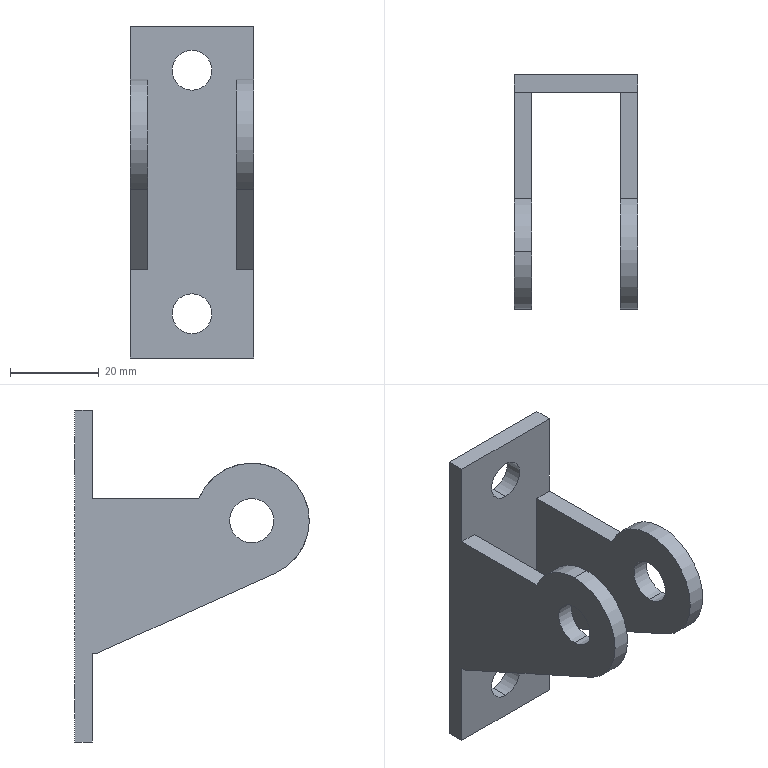Part | SolidWorks | features BaseBody 1 | 1 solid | 25 faces | box 28 x 53 x 75 mm | volume 17835 mm3 | plane 14 | cylinder 11 | commonest cylinder face diameters 9 x4 10 x4 26 x3
STEP:
#1=CARTESIAN_POINT('',(-400.,2358.,-1337.));
#2=VERTEX_POINT('',#1);
#3=CARTESIAN_POINT('',(-400.,2358.,-1328.));
#4=VERTEX_POINT('',#3);
#5=CARTESIAN_POINT('',(-400.,2358.,-1332.5));
#6=DIRECTION('',(0.,1.,0.));
#7=DIRECTION('',(0.,0.,1.));
#8=AXIS2_PLACEMENT_3D('',#5,#6,#7);
#9=CIRCLE('',#8,4.5);
#10=EDGE_CURVE('',#2,#4,#9,.T.);
#11=ORIENTED_EDGE('',*,*,#10,.F.);
#12=CARTESIAN_POINT('',(-400.,2362.,-1337.));
#13=VERTEX_POINT('',#12);
#14=CARTESIAN_POINT('',(-400.,2362.,-1337.));
#15=DIRECTION('',(0.,1.,0.));
#16=VECTOR('',#15,1000.);
#17=LINE('',#14,#16);
#18=EDGE_CURVE('',#2,#13,#17,.T.);
#19=ORIENTED_EDGE('',*,*,#18,.T.);
#20=CARTESIAN_POINT('',(-400.,2362.,-1328.));
#21=VERTEX_POINT('',#20);
#22=CARTESIAN_POINT('',(-400.,2362.,-1332.5));
#23=DIRECTION('',(0.,1.,0.));
#24=DIRECTION('',(0.,0.,1.));
#25=AXIS2_PLACEMENT_3D('',#22,#23,#24);
#26=CIRCLE('',#25,4.5);
#27=EDGE_CURVE('',#13,#21,#26,.T.);
#28=ORIENTED_EDGE('',*,*,#27,.T.);
#29=CARTESIAN_POINT('',(-400.,2362.,-1328.));
#30=DIRECTION('',(0.,1.,0.));
#31=VECTOR('',#30,1000.);
#32=LINE('',#29,#31);
#33=EDGE_CURVE('',#4,#21,#32,.T.);
#34=ORIENTED_EDGE('',*,*,#33,.F.);
#35=EDGE_LOOP('',(#11,#19,#28,#34));
#36=FACE_OUTER_BOUND('',#35,.T.);
#37=CARTESIAN_POINT('',(-400.,2362.,-1332.5));
#38=DIRECTION('',(0.,1.,0.));
#39=DIRECTION('',(0.,0.,1.));
#40=AXIS2_PLACEMENT_3D('',#37,#38,#39);
#41=CYLINDRICAL_SURFACE('',#40,4.5);
#42=ADVANCED_FACE('',(#36),#41,.F.);
#43=CARTESIAN_POINT('',(-400.,2362.,-1282.));
#44=VERTEX_POINT('',#43);
#45=CARTESIAN_POINT('',(-400.,2362.,-1273.));
#46=VERTEX_POINT('',#45);
#47=CARTESIAN_POINT('',(-400.,2362.,-1277.5));
#48=DIRECTION('',(0.,1.,0.));
#49=DIRECTION('',(0.,0.,-1.));
#50=AXIS2_PLACEMENT_3D('',#47,#48,#49);
#51=CIRCLE('',#50,4.5);
#52=EDGE_CURVE('',#44,#46,#51,.T.);
#53=ORIENTED_EDGE('',*,*,#52,.T.);
#54=CARTESIAN_POINT('',(-400.,2358.,-1273.));
#55=VERTEX_POINT('',#54);
#56=CARTESIAN_POINT('',(-400.,2362.,-1273.));
#57=DIRECTION('',(0.,-1.,0.));
#58=VECTOR('',#57,1000.);
#59=LINE('',#56,#58);
#60=EDGE_CURVE('',#46,#55,#59,.T.);
#61=ORIENTED_EDGE('',*,*,#60,.T.);
#62=CARTESIAN_POINT('',(-400.,2358.,-1282.));
#63=VERTEX_POINT('',#62);
#64=CARTESIAN_POINT('',(-400.,2358.,-1277.5));
#65=DIRECTION('',(0.,1.,0.));
#66=DIRECTION('',(0.,0.,-1.));
#67=AXIS2_PLACEMENT_3D('',#64,#65,#66);
#68=CIRCLE('',#67,4.5);
#69=EDGE_CURVE('',#63,#55,#68,.T.);
#70=ORIENTED_EDGE('',*,*,#69,.F.);
#71=CARTESIAN_POINT('',(-400.,2362.,-1282.));
#72=DIRECTION('',(0.,-1.,0.));
#73=VECTOR('',#72,1000.);
#74=LINE('',#71,#73);
#75=EDGE_CURVE('',#44,#63,#74,.T.);
#76=ORIENTED_EDGE('',*,*,#75,.F.);
#77=EDGE_LOOP('',(#53,#61,#70,#76));
#78=FACE_OUTER_BOUND('',#77,.T.);
#79=CARTESIAN_POINT('',(-400.,2362.,-1277.5));
#80=DIRECTION('',(0.,-1.,0.));
#81=DIRECTION('',(0.,0.,-1.));
#82=AXIS2_PLACEMENT_3D('',#79,#80,#81);
#83=CYLINDRICAL_SURFACE('',#82,4.5);
#84=ADVANCED_FACE('',(#78),#83,.F.);
#85=CARTESIAN_POINT('',(-410.,2322.,-1297.5));
#86=VERTEX_POINT('',#85);
#87=CARTESIAN_POINT('',(-410.,2322.,-1287.5));
#88=VERTEX_POINT('',#87);
#89=CARTESIAN_POINT('',(-410.,2322.,-1292.5));
#90=DIRECTION('',(-1.,0.,0.));
#91=DIRECTION('',(0.,0.,1.));
#92=AXIS2_PLACEMENT_3D('',#89,#90,#91);
#93=CIRCLE('',#92,5.);
#94=EDGE_CURVE('',#86,#88,#93,.T.);
#95=ORIENTED_EDGE('',*,*,#94,.F.);
#96=CARTESIAN_POINT('',(-414.,2322.,-1297.5));
#97=VERTEX_POINT('',#96);
#98=CARTESIAN_POINT('',(-414.,2322.,-1297.5));
#99=DIRECTION('',(-1.,0.,0.));
#100=VECTOR('',#99,1000.);
#101=LINE('',#98,#100);
#102=EDGE_CURVE('',#86,#97,#101,.T.);
#103=ORIENTED_EDGE('',*,*,#102,.T.);
#104=CARTESIAN_POINT('',(-414.,2322.,-1287.5));
#105=VERTEX_POINT('',#104);
#106=CARTESIAN_POINT('',(-414.,2322.,-1292.5));
#107=DIRECTION('',(1.,0.,0.));
#108=DIRECTION('',(0.,0.,1.));
#109=AXIS2_PLACEMENT_3D('',#106,#107,#108);
#110=CIRCLE('',#109,5.);
#111=EDGE_CURVE('',#105,#97,#110,.T.);
#112=ORIENTED_EDGE('',*,*,#111,.F.);
#113=CARTESIAN_POINT('',(-414.,2322.,-1287.5));
#114=DIRECTION('',(-1.,0.,0.));
#115=VECTOR('',#114,1000.);
#116=LINE('',#113,#115);
#117=EDGE_CURVE('',#88,#105,#116,.T.);
#118=ORIENTED_EDGE('',*,*,#117,.F.);
#119=EDGE_LOOP('',(#95,#103,#112,#118));
#120=FACE_OUTER_BOUND('',#119,.T.);
#121=CARTESIAN_POINT('',(-414.,2322.,-1292.5));
#122=DIRECTION('',(-1.,0.,0.));
#123=DIRECTION('',(0.,0.,1.));
#124=AXIS2_PLACEMENT_3D('',#121,#122,#123);
#125=CYLINDRICAL_SURFACE('',#124,5.);
#126=ADVANCED_FACE('',(#120),#125,.F.);
#127=CARTESIAN_POINT('',(-410.,2316.667,-1304.356));
#128=VERTEX_POINT('',#127);
#129=CARTESIAN_POINT('',(-410.,2322.,-1279.5));
#130=VERTEX_POINT('',#129);
#131=CARTESIAN_POINT('',(-410.,2322.,-1292.5));
#132=DIRECTION('',(-1.,0.,0.));
#133=DIRECTION('',(0.,0.,1.));
#134=AXIS2_PLACEMENT_3D('',#131,#132,#133);
#135=CIRCLE('',#134,13.);
#136=EDGE_CURVE('',#128,#130,#135,.T.);
#137=ORIENTED_EDGE('',*,*,#136,.T.);
#138=CARTESIAN_POINT('',(-414.,2322.,-1279.5));
#139=VERTEX_POINT('',#138);
#140=CARTESIAN_POINT('',(-414.,2322.,-1279.5));
#141=DIRECTION('',(-1.,0.,0.));
#142=VECTOR('',#141,1000.);
#143=LINE('',#140,#142);
#144=EDGE_CURVE('',#130,#139,#143,.T.);
#145=ORIENTED_EDGE('',*,*,#144,.T.);
#146=CARTESIAN_POINT('',(-414.,2316.667,-1304.356));
#147=VERTEX_POINT('',#146);
#148=CARTESIAN_POINT('',(-414.,2322.,-1292.5));
#149=DIRECTION('',(-1.,0.,0.));
#150=DIRECTION('',(0.,0.,1.));
#151=AXIS2_PLACEMENT_3D('',#148,#149,#150);
#152=CIRCLE('',#151,13.);
#153=EDGE_CURVE('',#147,#139,#152,.T.);
#154=ORIENTED_EDGE('',*,*,#153,.F.);
#155=CARTESIAN_POINT('',(-414.,2316.667,-1304.356));
#156=DIRECTION('',(1.,0.,0.));
#157=VECTOR('',#156,1000.);
#158=LINE('',#155,#157);
#159=EDGE_CURVE('',#147,#128,#158,.T.);
#160=ORIENTED_EDGE('',*,*,#159,.T.);
#161=EDGE_LOOP('',(#137,#145,#154,#160));
#162=FACE_OUTER_BOUND('',#161,.T.);
#163=CARTESIAN_POINT('',(-414.,2322.,-1292.5));
#164=DIRECTION('',(-1.,0.,0.));
#165=DIRECTION('',(0.,0.,1.));
#166=AXIS2_PLACEMENT_3D('',#163,#164,#165);
#167=CYLINDRICAL_SURFACE('',#166,13.);
#168=ADVANCED_FACE('',(#162),#167,.T.);
#169=CARTESIAN_POINT('',(-390.,2322.,-1287.5));
#170=VERTEX_POINT('',#169);
#171=CARTESIAN_POINT('',(-390.,2322.,-1297.5));
#172=VERTEX_POINT('',#171);
#173=CARTESIAN_POINT('',(-390.,2322.,-1292.5));
#174=DIRECTION('',(1.,0.,0.));
#175=DIRECTION('',(0.,0.,-1.));
#176=AXIS2_PLACEMENT_3D('',#173,#174,#175);
#177=CIRCLE('',#176,5.);
#178=EDGE_CURVE('',#170,#172,#177,.T.);
#179=ORIENTED_EDGE('',*,*,#178,.F.);
#180=CARTESIAN_POINT('',(-386.,2322.,-1287.5));
#181=VERTEX_POINT('',#180);
#182=CARTESIAN_POINT('',(-386.,2322.,-1287.5));
#183=DIRECTION('',(1.,0.,0.));
#184=VECTOR('',#183,1000.);
#185=LINE('',#182,#184);
#186=EDGE_CURVE('',#170,#181,#185,.T.);
#187=ORIENTED_EDGE('',*,*,#186,.T.);
#188=CARTESIAN_POINT('',(-386.,2322.,-1297.5));
#189=VERTEX_POINT('',#188);
#190=CARTESIAN_POINT('',(-386.,2322.,-1292.5));
#191=DIRECTION('',(-1.,0.,0.));
#192=DIRECTION('',(0.,0.,-1.));
#193=AXIS2_PLACEMENT_3D('',#190,#191,#192);
#194=CIRCLE('',#193,5.);
#195=EDGE_CURVE('',#189,#181,#194,.T.);
#196=ORIENTED_EDGE('',*,*,#195,.F.);
#197=CARTESIAN_POINT('',(-386.,2322.,-1297.5));
#198=DIRECTION('',(1.,0.,0.));
#199=VECTOR('',#198,1000.);
#200=LINE('',#197,#199);
#201=EDGE_CURVE('',#172,#189,#200,.T.);
#202=ORIENTED_EDGE('',*,*,#201,.F.);
#203=EDGE_LOOP('',(#179,#187,#196,#202));
#204=FACE_OUTER_BOUND('',#203,.T.);
#205=CARTESIAN_POINT('',(-386.,2322.,-1292.5));
#206=DIRECTION('',(1.,0.,0.));
#207=DIRECTION('',(0.,0.,-1.));
#208=AXIS2_PLACEMENT_3D('',#205,#206,#207);
#209=CYLINDRICAL_SURFACE('',#208,5.);
#210=ADVANCED_FACE('',(#204),#209,.F.);
#211=CARTESIAN_POINT('',(-400.,2362.,-1332.5));
#212=DIRECTION('',(0.,1.,0.));
#213=DIRECTION('',(0.,0.,1.));
#214=AXIS2_PLACEMENT_3D('',#211,#212,#213);
#215=CIRCLE('',#214,4.5);
#216=EDGE_CURVE('',#21,#13,#215,.T.);
#217=ORIENTED_EDGE('',*,*,#216,.F.);
#218=ORIENTED_EDGE('',*,*,#27,.F.);
#219=EDGE_LOOP('',(#217,#218));
#220=FACE_BOUND('',#219,.T.);
#221=ORIENTED_EDGE('',*,*,#52,.F.);
#222=CARTESIAN_POINT('',(-400.,2362.,-1277.5));
#223=DIRECTION('',(0.,1.,0.));
#224=DIRECTION('',(0.,0.,-1.));
#225=AXIS2_PLACEMENT_3D('',#222,#223,#224);
#226=CIRCLE('',#225,4.5);
#227=EDGE_CURVE('',#46,#44,#226,.T.);
#228=ORIENTED_EDGE('',*,*,#227,.F.);
#229=EDGE_LOOP('',(#221,#228));
#230=FACE_BOUND('',#229,.T.);
#231=CARTESIAN_POINT('',(-386.,2362.,-1267.5));
#232=VERTEX_POINT('',#231);
#233=CARTESIAN_POINT('',(-414.,2362.,-1267.5));
#234=VERTEX_POINT('',#233);
#235=CARTESIAN_POINT('',(-400.,2362.,-1267.5));
#236=DIRECTION('',(-1.,0.,0.));
#237=VECTOR('',#236,1000.);
#238=LINE('',#235,#237);
#239=EDGE_CURVE('',#232,#234,#238,.T.);
#240=ORIENTED_EDGE('',*,*,#239,.F.);
#241=CARTESIAN_POINT('',(-386.,2362.,-1342.5));
#242=VERTEX_POINT('',#241);
#243=CARTESIAN_POINT('',(-386.,2362.,-1292.5));
#244=DIRECTION('',(0.,0.,1.));
#245=VECTOR('',#244,1000.);
#246=LINE('',#243,#245);
#247=EDGE_CURVE('',#242,#232,#246,.T.);
#248=ORIENTED_EDGE('',*,*,#247,.F.);
#249=CARTESIAN_POINT('',(-414.,2362.,-1342.5));
#250=VERTEX_POINT('',#249);
#251=CARTESIAN_POINT('',(-400.,2362.,-1342.5));
#252=DIRECTION('',(1.,0.,0.));
#253=VECTOR('',#252,1000.);
#254=LINE('',#251,#253);
#255=EDGE_CURVE('',#250,#242,#254,.T.);
#256=ORIENTED_EDGE('',*,*,#255,.F.);
#257=CARTESIAN_POINT('',(-414.,2362.,-1292.5));
#258=DIRECTION('',(0.,0.,-1.));
#259=VECTOR('',#258,1000.);
#260=LINE('',#257,#259);
#261=EDGE_CURVE('',#234,#250,#260,.T.);
#262=ORIENTED_EDGE('',*,*,#261,.F.);
#263=EDGE_LOOP('',(#240,#248,#256,#262));
#264=FACE_OUTER_BOUND('',#263,.T.);
#265=CARTESIAN_POINT('',(-400.,2362.,-1292.5));
#266=DIRECTION('',(0.,-1.,0.));
#267=DIRECTION('',(0.,0.,-1.));
#268=AXIS2_PLACEMENT_3D('',#265,#266,#267);
#269=PLANE('',#268);
#270=ADVANCED_FACE('',(#220,#230,#264),#269,.F.);
#271=ORIENTED_EDGE('',*,*,#18,.F.);
#272=CARTESIAN_POINT('',(-400.,2358.,-1332.5));
#273=DIRECTION('',(0.,1.,0.));
#274=DIRECTION('',(0.,0.,1.));
#275=AXIS2_PLACEMENT_3D('',#272,#273,#274);
#276=CIRCLE('',#275,4.5);
#277=EDGE_CURVE('',#4,#2,#276,.T.);
#278=ORIENTED_EDGE('',*,*,#277,.F.);
#279=ORIENTED_EDGE('',*,*,#33,.T.);
#280=ORIENTED_EDGE('',*,*,#216,.T.);
#281=EDGE_LOOP('',(#271,#278,#279,#280));
#282=FACE_OUTER_BOUND('',#281,.T.);
#283=CARTESIAN_POINT('',(-400.,2362.,-1332.5));
#284=DIRECTION('',(0.,1.,0.));
#285=DIRECTION('',(0.,0.,1.));
#286=AXIS2_PLACEMENT_3D('',#283,#284,#285);
#287=CYLINDRICAL_SURFACE('',#286,4.5);
#288=ADVANCED_FACE('',(#282),#287,.F.);
#289=ORIENTED_EDGE('',*,*,#60,.F.);
#290=ORIENTED_EDGE('',*,*,#227,.T.);
#291=ORIENTED_EDGE('',*,*,#75,.T.);
#292=CARTESIAN_POINT('',(-400.,2358.,-1277.5));
#293=DIRECTION('',(0.,1.,0.));
#294=DIRECTION('',(0.,0.,-1.));
#295=AXIS2_PLACEMENT_3D('',#292,#293,#294);
#296=CIRCLE('',#295,4.5);
#297=EDGE_CURVE('',#55,#63,#296,.T.);
#298=ORIENTED_EDGE('',*,*,#297,.F.);
#299=EDGE_LOOP('',(#289,#290,#291,#298));
#300=FACE_OUTER_BOUND('',#299,.T.);
#301=CARTESIAN_POINT('',(-400.,2362.,-1277.5));
#302=DIRECTION('',(0.,-1.,0.));
#303=DIRECTION('',(0.,0.,-1.));
#304=AXIS2_PLACEMENT_3D('',#301,#302,#303);
#305=CYLINDRICAL_SURFACE('',#304,4.5);
#306=ADVANCED_FACE('',(#300),#305,.F.);
#307=ORIENTED_EDGE('',*,*,#111,.T.);
#308=CARTESIAN_POINT('',(-414.,2322.,-1292.5));
#309=DIRECTION('',(1.,0.,0.));
#310=DIRECTION('',(0.,0.,1.));
#311=AXIS2_PLACEMENT_3D('',#308,#309,#310);
#312=CIRCLE('',#311,5.);
#313=EDGE_CURVE('',#97,#105,#312,.T.);
#314=ORIENTED_EDGE('',*,*,#313,.T.);
#315=EDGE_LOOP('',(#307,#314));
#316=FACE_BOUND('',#315,.T.);
#317=CARTESIAN_POINT('',(-414.,2334.,-1287.5));
#318=VERTEX_POINT('',#317);
#319=CARTESIAN_POINT('',(-414.,2358.,-1287.5));
#320=VERTEX_POINT('',#319);
#321=CARTESIAN_POINT('',(-414.,2362.,-1287.5));
#322=DIRECTION('',(0.,1.,0.));
#323=VECTOR('',#322,1000.);
#324=LINE('',#321,#323);
#325=EDGE_CURVE('',#318,#320,#324,.T.);
#326=ORIENTED_EDGE('',*,*,#325,.T.);
#327=CARTESIAN_POINT('',(-414.,2358.,-1267.5));
#328=VERTEX_POINT('',#327);
#329=CARTESIAN_POINT('',(-414.,2358.,-1342.5));
#330=DIRECTION('',(0.,0.,1.));
#331=VECTOR('',#330,1000.);
#332=LINE('',#329,#331);
#333=EDGE_CURVE('',#320,#328,#332,.T.);
#334=ORIENTED_EDGE('',*,*,#333,.T.);
#335=CARTESIAN_POINT('',(-414.,2362.,-1267.5));
#336=DIRECTION('',(0.,1.,0.));
#337=VECTOR('',#336,1000.);
#338=LINE('',#335,#337);
#339=EDGE_CURVE('',#328,#234,#338,.T.);
#340=ORIENTED_EDGE('',*,*,#339,.T.);
#341=ORIENTED_EDGE('',*,*,#261,.T.);
#342=CARTESIAN_POINT('',(-414.,2358.,-1342.5));
#343=VERTEX_POINT('',#342);
#344=CARTESIAN_POINT('',(-414.,2362.,-1342.5));
#345=DIRECTION('',(0.,-1.,0.));
#346=VECTOR('',#345,1000.);
#347=LINE('',#344,#346);
#348=EDGE_CURVE('',#250,#343,#347,.T.);
#349=ORIENTED_EDGE('',*,*,#348,.T.);
#350=CARTESIAN_POINT('',(-414.,2358.,-1322.5));
#351=VERTEX_POINT('',#350);
#352=CARTESIAN_POINT('',(-414.,2358.,-1342.5));
#353=DIRECTION('',(0.,0.,1.));
#354=VECTOR('',#353,1000.);
#355=LINE('',#352,#354);
#356=EDGE_CURVE('',#343,#351,#355,.T.);
#357=ORIENTED_EDGE('',*,*,#356,.T.);
#358=CARTESIAN_POINT('',(-414.,2357.,-1322.5));
#359=VERTEX_POINT('',#358);
#360=CARTESIAN_POINT('',(-414.,2362.,-1322.5));
#361=DIRECTION('',(0.,-1.,0.));
#362=VECTOR('',#361,1000.);
#363=LINE('',#360,#362);
#364=EDGE_CURVE('',#351,#359,#363,.T.);
#365=ORIENTED_EDGE('',*,*,#364,.T.);
#366=CARTESIAN_POINT('',(-414.,2357.,-1322.5));
#367=DIRECTION('',(0.,-0.912,0.4103));
#368=VECTOR('',#367,1000.);
#369=LINE('',#366,#368);
#370=EDGE_CURVE('',#359,#147,#369,.T.);
#371=ORIENTED_EDGE('',*,*,#370,.T.);
#372=ORIENTED_EDGE('',*,*,#153,.T.);
#373=CARTESIAN_POINT('',(-414.,2322.,-1292.5));
#374=DIRECTION('',(-1.,0.,0.));
#375=DIRECTION('',(0.,0.,1.));
#376=AXIS2_PLACEMENT_3D('',#373,#374,#375);
#377=CIRCLE('',#376,13.);
#378=EDGE_CURVE('',#139,#318,#377,.T.);
#379=ORIENTED_EDGE('',*,*,#378,.T.);
#380=EDGE_LOOP('',(#326,#334,#340,#341,#349,#357,#365,#371,#372,#379));
#381=FACE_OUTER_BOUND('',#380,.T.);
#382=CARTESIAN_POINT('',(-414.,2362.,-1342.5));
#383=DIRECTION('',(-1.,0.,0.));
#384=DIRECTION('',(0.,0.,1.));
#385=AXIS2_PLACEMENT_3D('',#382,#383,#384);
#386=PLANE('',#385);
#387=ADVANCED_FACE('',(#316,#381),#386,.T.);
#388=CARTESIAN_POINT('',(-386.,2358.,-1267.5));
#389=VERTEX_POINT('',#388);
#390=CARTESIAN_POINT('',(-386.,2362.,-1267.5));
#391=DIRECTION('',(0.,1.,0.));
#392=VECTOR('',#391,1000.);
#393=LINE('',#390,#392);
#394=EDGE_CURVE('',#389,#232,#393,.T.);
#395=ORIENTED_EDGE('',*,*,#394,.T.);
#396=ORIENTED_EDGE('',*,*,#239,.T.);
#397=ORIENTED_EDGE('',*,*,#339,.F.);
#398=CARTESIAN_POINT('',(-414.,2358.,-1267.5));
#399=DIRECTION('',(1.,0.,0.));
#400=VECTOR('',#399,1000.);
#401=LINE('',#398,#400);
#402=EDGE_CURVE('',#328,#389,#401,.T.);
#403=ORIENTED_EDGE('',*,*,#402,.T.);
#404=EDGE_LOOP('',(#395,#396,#397,#403));
#405=FACE_OUTER_BOUND('',#404,.T.);
#406=CARTESIAN_POINT('',(-414.,2362.,-1267.5));
#407=DIRECTION('',(0.,0.,1.));
#408=DIRECTION('',(1.,0.,0.));
#409=AXIS2_PLACEMENT_3D('',#406,#407,#408);
#410=PLANE('',#409);
#411=ADVANCED_FACE('',(#405),#410,.T.);
#412=ORIENTED_EDGE('',*,*,#195,.T.);
#413=CARTESIAN_POINT('',(-386.,2322.,-1292.5));
#414=DIRECTION('',(-1.,0.,0.));
#415=DIRECTION('',(0.,0.,-1.));
#416=AXIS2_PLACEMENT_3D('',#413,#414,#415);
#417=CIRCLE('',#416,5.);
#418=EDGE_CURVE('',#181,#189,#417,.T.);
#419=ORIENTED_EDGE('',*,*,#418,.T.);
#420=EDGE_LOOP('',(#412,#419));
#421=FACE_BOUND('',#420,.T.);
#422=CARTESIAN_POINT('',(-386.,2357.,-1322.5));
#423=VERTEX_POINT('',#422);
#424=CARTESIAN_POINT('',(-386.,2358.,-1322.5));
#425=VERTEX_POINT('',#424);
#426=CARTESIAN_POINT('',(-386.,2362.,-1322.5));
#427=DIRECTION('',(0.,1.,0.));
#428=VECTOR('',#427,1000.);
#429=LINE('',#426,#428);
#430=EDGE_CURVE('',#423,#425,#429,.T.);
#431=ORIENTED_EDGE('',*,*,#430,.T.);
#432=CARTESIAN_POINT('',(-386.,2358.,-1342.5));
#433=VERTEX_POINT('',#432);
#434=CARTESIAN_POINT('',(-386.,2358.,-1267.5));
#435=DIRECTION('',(0.,0.,-1.));
#436=VECTOR('',#435,1000.);
#437=LINE('',#434,#436);
#438=EDGE_CURVE('',#425,#433,#437,.T.);
#439=ORIENTED_EDGE('',*,*,#438,.T.);
#440=CARTESIAN_POINT('',(-386.,2362.,-1342.5));
#441=DIRECTION('',(0.,1.,0.));
#442=VECTOR('',#441,1000.);
#443=LINE('',#440,#442);
#444=EDGE_CURVE('',#433,#242,#443,.T.);
#445=ORIENTED_EDGE('',*,*,#444,.T.);
#446=ORIENTED_EDGE('',*,*,#247,.T.);
#447=ORIENTED_EDGE('',*,*,#394,.F.);
#448=CARTESIAN_POINT('',(-386.,2358.,-1287.5));
#449=VERTEX_POINT('',#448);
#450=CARTESIAN_POINT('',(-386.,2358.,-1267.5));
#451=DIRECTION('',(0.,0.,-1.));
#452=VECTOR('',#451,1000.);
#453=LINE('',#450,#452);
#454=EDGE_CURVE('',#389,#449,#453,.T.);
#455=ORIENTED_EDGE('',*,*,#454,.T.);
#456=CARTESIAN_POINT('',(-386.,2334.,-1287.5));
#457=VERTEX_POINT('',#456);
#458=CARTESIAN_POINT('',(-386.,2362.,-1287.5));
#459=DIRECTION('',(0.,-1.,0.));
#460=VECTOR('',#459,1000.);
#461=LINE('',#458,#460);
#462=EDGE_CURVE('',#449,#457,#461,.T.);
#463=ORIENTED_EDGE('',*,*,#462,.T.);
#464=CARTESIAN_POINT('',(-386.,2316.667,-1304.356));
#465=VERTEX_POINT('',#464);
#466=CARTESIAN_POINT('',(-386.,2322.,-1292.5));
#467=DIRECTION('',(1.,0.,0.));
#468=DIRECTION('',(0.,0.,-1.));
#469=AXIS2_PLACEMENT_3D('',#466,#467,#468);
#470=CIRCLE('',#469,13.);
#471=EDGE_CURVE('',#457,#465,#470,.T.);
#472=ORIENTED_EDGE('',*,*,#471,.T.);
#473=CARTESIAN_POINT('',(-386.,2316.667,-1304.356));
#474=DIRECTION('',(0.,0.912,-0.4103));
#475=VECTOR('',#474,1000.);
#476=LINE('',#473,#475);
#477=EDGE_CURVE('',#465,#423,#476,.T.);
#478=ORIENTED_EDGE('',*,*,#477,.T.);
#479=EDGE_LOOP('',(#431,#439,#445,#446,#447,#455,#463,#472,#478));
#480=FACE_OUTER_BOUND('',#479,.T.);
#481=CARTESIAN_POINT('',(-386.,2362.,-1267.5));
#482=DIRECTION('',(1.,0.,0.));
#483=DIRECTION('',(0.,0.,-1.));
#484=AXIS2_PLACEMENT_3D('',#481,#482,#483);
#485=PLANE('',#484);
#486=ADVANCED_FACE('',(#421,#480),#485,.T.);
#487=ORIENTED_EDGE('',*,*,#348,.F.);
#488=ORIENTED_EDGE('',*,*,#255,.T.);
#489=ORIENTED_EDGE('',*,*,#444,.F.);
#490=CARTESIAN_POINT('',(-386.,2358.,-1342.5));
#491=DIRECTION('',(-1.,0.,0.));
#492=VECTOR('',#491,1000.);
#493=LINE('',#490,#492);
#494=EDGE_CURVE('',#433,#343,#493,.T.);
#495=ORIENTED_EDGE('',*,*,#494,.T.);
#496=EDGE_LOOP('',(#487,#488,#489,#495));
#497=FACE_OUTER_BOUND('',#496,.T.);
#498=CARTESIAN_POINT('',(-386.,2362.,-1342.5));
#499=DIRECTION('',(0.,0.,-1.));
#500=DIRECTION('',(-1.,0.,0.));
#501=AXIS2_PLACEMENT_3D('',#498,#499,#500);
#502=PLANE('',#501);
#503=ADVANCED_FACE('',(#497),#502,.T.);
#504=ORIENTED_EDGE('',*,*,#277,.T.);
#505=ORIENTED_EDGE('',*,*,#10,.T.);
#506=EDGE_LOOP('',(#504,#505));
#507=FACE_BOUND('',#506,.T.);
#508=ORIENTED_EDGE('',*,*,#69,.T.);
#509=ORIENTED_EDGE('',*,*,#297,.T.);
#510=EDGE_LOOP('',(#508,#509));
#511=FACE_BOUND('',#510,.T.);
#512=ORIENTED_EDGE('',*,*,#438,.F.);
#513=CARTESIAN_POINT('',(-390.,2358.,-1322.5));
#514=VERTEX_POINT('',#513);
#515=CARTESIAN_POINT('',(-400.,2358.,-1322.5));
#516=DIRECTION('',(-1.,0.,0.));
#517=VECTOR('',#516,1000.);
#518=LINE('',#515,#517);
#519=EDGE_CURVE('',#425,#514,#518,.T.);
#520=ORIENTED_EDGE('',*,*,#519,.T.);
#521=CARTESIAN_POINT('',(-390.,2358.,-1287.5));
#522=VERTEX_POINT('',#521);
#523=CARTESIAN_POINT('',(-390.,2358.,-1292.5));
#524=DIRECTION('',(0.,0.,1.));
#525=VECTOR('',#524,1000.);
#526=LINE('',#523,#525);
#527=EDGE_CURVE('',#514,#522,#526,.T.);
#528=ORIENTED_EDGE('',*,*,#527,.T.);
#529=CARTESIAN_POINT('',(-400.,2358.,-1287.5));
#530=DIRECTION('',(1.,0.,0.));
#531=VECTOR('',#530,1000.);
#532=LINE('',#529,#531);
#533=EDGE_CURVE('',#522,#449,#532,.T.);
#534=ORIENTED_EDGE('',*,*,#533,.T.);
#535=ORIENTED_EDGE('',*,*,#454,.F.);
#536=ORIENTED_EDGE('',*,*,#402,.F.);
#537=ORIENTED_EDGE('',*,*,#333,.F.);
#538=CARTESIAN_POINT('',(-410.,2358.,-1287.5));
#539=VERTEX_POINT('',#538);
#540=CARTESIAN_POINT('',(-400.,2358.,-1287.5));
#541=DIRECTION('',(1.,0.,0.));
#542=VECTOR('',#541,1000.);
#543=LINE('',#540,#542);
#544=EDGE_CURVE('',#320,#539,#543,.T.);
#545=ORIENTED_EDGE('',*,*,#544,.T.);
#546=CARTESIAN_POINT('',(-410.,2358.,-1322.5));
#547=VERTEX_POINT('',#546);
#548=CARTESIAN_POINT('',(-410.,2358.,-1292.5));
#549=DIRECTION('',(0.,0.,-1.));
#550=VECTOR('',#549,1000.);
#551=LINE('',#548,#550);
#552=EDGE_CURVE('',#539,#547,#551,.T.);
#553=ORIENTED_EDGE('',*,*,#552,.T.);
#554=CARTESIAN_POINT('',(-400.,2358.,-1322.5));
#555=DIRECTION('',(-1.,0.,0.));
#556=VECTOR('',#555,1000.);
#557=LINE('',#554,#556);
#558=EDGE_CURVE('',#547,#351,#557,.T.);
#559=ORIENTED_EDGE('',*,*,#558,.T.);
#560=ORIENTED_EDGE('',*,*,#356,.F.);
#561=ORIENTED_EDGE('',*,*,#494,.F.);
#562=EDGE_LOOP('',(#512,#520,#528,#534,#535,#536,#537,#545,#553,#559,#560,#561));
#563=FACE_OUTER_BOUND('',#562,.T.);
#564=CARTESIAN_POINT('',(-400.,2358.,-1292.5));
#565=DIRECTION('',(0.,-1.,0.));
#566=DIRECTION('',(0.,0.,-1.));
#567=AXIS2_PLACEMENT_3D('',#564,#565,#566);
#568=PLANE('',#567);
#569=ADVANCED_FACE('',(#507,#511,#563),#568,.T.);
#570=ORIENTED_EDGE('',*,*,#102,.F.);
#571=CARTESIAN_POINT('',(-410.,2322.,-1292.5));
#572=DIRECTION('',(-1.,0.,0.));
#573=DIRECTION('',(0.,0.,1.));
#574=AXIS2_PLACEMENT_3D('',#571,#572,#573);
#575=CIRCLE('',#574,5.);
#576=EDGE_CURVE('',#88,#86,#575,.T.);
#577=ORIENTED_EDGE('',*,*,#576,.F.);
#578=ORIENTED_EDGE('',*,*,#117,.T.);
#579=ORIENTED_EDGE('',*,*,#313,.F.);
#580=EDGE_LOOP('',(#570,#577,#578,#579));
#581=FACE_OUTER_BOUND('',#580,.T.);
#582=CARTESIAN_POINT('',(-414.,2322.,-1292.5));
#583=DIRECTION('',(-1.,0.,0.));
#584=DIRECTION('',(0.,0.,1.));
#585=AXIS2_PLACEMENT_3D('',#582,#583,#584);
#586=CYLINDRICAL_SURFACE('',#585,5.);
#587=ADVANCED_FACE('',(#581),#586,.F.);
#588=ORIENTED_EDGE('',*,*,#325,.F.);
#589=CARTESIAN_POINT('',(-410.,2334.,-1287.5));
#590=VERTEX_POINT('',#589);
#591=CARTESIAN_POINT('',(-414.,2334.,-1287.5));
#592=DIRECTION('',(1.,0.,0.));
#593=VECTOR('',#592,1000.);
#594=LINE('',#591,#593);
#595=EDGE_CURVE('',#318,#590,#594,.T.);
#596=ORIENTED_EDGE('',*,*,#595,.T.);
#597=CARTESIAN_POINT('',(-410.,2334.,-1287.5));
#598=DIRECTION('',(0.,1.,0.));
#599=VECTOR('',#598,1000.);
#600=LINE('',#597,#599);
#601=EDGE_CURVE('',#590,#539,#600,.T.);
#602=ORIENTED_EDGE('',*,*,#601,.T.);
#603=ORIENTED_EDGE('',*,*,#544,.F.);
#604=EDGE_LOOP('',(#588,#596,#602,#603));
#605=FACE_OUTER_BOUND('',#604,.T.);
#606=CARTESIAN_POINT('',(-414.,2334.,-1287.5));
#607=DIRECTION('',(0.,0.,1.));
#608=DIRECTION('',(1.,0.,0.));
#609=AXIS2_PLACEMENT_3D('',#606,#607,#608);
#610=PLANE('',#609);
#611=ADVANCED_FACE('',(#605),#610,.T.);
#612=ORIENTED_EDGE('',*,*,#144,.F.);
#613=CARTESIAN_POINT('',(-410.,2322.,-1292.5));
#614=DIRECTION('',(-1.,0.,0.));
#615=DIRECTION('',(0.,0.,1.));
#616=AXIS2_PLACEMENT_3D('',#613,#614,#615);
#617=CIRCLE('',#616,13.);
#618=EDGE_CURVE('',#130,#590,#617,.T.);
#619=ORIENTED_EDGE('',*,*,#618,.T.);
#620=ORIENTED_EDGE('',*,*,#595,.F.);
#621=ORIENTED_EDGE('',*,*,#378,.F.);
#622=EDGE_LOOP('',(#612,#619,#620,#621));
#623=FACE_OUTER_BOUND('',#622,.T.);
#624=CARTESIAN_POINT('',(-414.,2322.,-1292.5));
#625=DIRECTION('',(-1.,0.,0.));
#626=DIRECTION('',(0.,0.,1.));
#627=AXIS2_PLACEMENT_3D('',#624,#625,#626);
#628=CYLINDRICAL_SURFACE('',#627,13.);
#629=ADVANCED_FACE('',(#623),#628,.T.);
#630=ORIENTED_EDGE('',*,*,#159,.F.);
#631=ORIENTED_EDGE('',*,*,#370,.F.);
#632=CARTESIAN_POINT('',(-410.,2357.,-1322.5));
#633=VERTEX_POINT('',#632);
#634=CARTESIAN_POINT('',(-414.,2357.,-1322.5));
#635=DIRECTION('',(1.,0.,0.));
#636=VECTOR('',#635,1000.);
#637=LINE('',#634,#636);
#638=EDGE_CURVE('',#359,#633,#637,.T.);
#639=ORIENTED_EDGE('',*,*,#638,.T.);
#640=CARTESIAN_POINT('',(-410.,2357.,-1322.5));
#641=DIRECTION('',(0.,-0.912,0.4103));
#642=VECTOR('',#641,1000.);
#643=LINE('',#640,#642);
#644=EDGE_CURVE('',#633,#128,#643,.T.);
#645=ORIENTED_EDGE('',*,*,#644,.T.);
#646=EDGE_LOOP('',(#630,#631,#639,#645));
#647=FACE_OUTER_BOUND('',#646,.T.);
#648=CARTESIAN_POINT('',(-414.,2357.,-1322.5));
#649=DIRECTION('',(0.,-0.4103,-0.912));
#650=DIRECTION('',(0.,0.912,-0.4103));
#651=AXIS2_PLACEMENT_3D('',#648,#649,#650);
#652=PLANE('',#651);
#653=ADVANCED_FACE('',(#647),#652,.T.);
#654=CARTESIAN_POINT('',(-410.,2362.,-1322.5));
#655=DIRECTION('',(0.,-1.,0.));
#656=VECTOR('',#655,1000.);
#657=LINE('',#654,#656);
#658=EDGE_CURVE('',#547,#633,#657,.T.);
#659=ORIENTED_EDGE('',*,*,#658,.T.);
#660=ORIENTED_EDGE('',*,*,#638,.F.);
#661=ORIENTED_EDGE('',*,*,#364,.F.);
#662=ORIENTED_EDGE('',*,*,#558,.F.);
#663=EDGE_LOOP('',(#659,#660,#661,#662));
#664=FACE_OUTER_BOUND('',#663,.T.);
#665=CARTESIAN_POINT('',(-414.,2362.,-1322.5));
#666=DIRECTION('',(0.,0.,-1.));
#667=DIRECTION('',(-1.,0.,0.));
#668=AXIS2_PLACEMENT_3D('',#665,#666,#667);
#669=PLANE('',#668);
#670=ADVANCED_FACE('',(#664),#669,.T.);
#671=ORIENTED_EDGE('',*,*,#186,.F.);
#672=CARTESIAN_POINT('',(-390.,2322.,-1292.5));
#673=DIRECTION('',(1.,0.,0.));
#674=DIRECTION('',(0.,0.,-1.));
#675=AXIS2_PLACEMENT_3D('',#672,#673,#674);
#676=CIRCLE('',#675,5.);
#677=EDGE_CURVE('',#172,#170,#676,.T.);
#678=ORIENTED_EDGE('',*,*,#677,.F.);
#679=ORIENTED_EDGE('',*,*,#201,.T.);
#680=ORIENTED_EDGE('',*,*,#418,.F.);
#681=EDGE_LOOP('',(#671,#678,#679,#680));
#682=FACE_OUTER_BOUND('',#681,.T.);
#683=CARTESIAN_POINT('',(-386.,2322.,-1292.5));
#684=DIRECTION('',(1.,0.,0.));
#685=DIRECTION('',(0.,0.,-1.));
#686=AXIS2_PLACEMENT_3D('',#683,#684,#685);
#687=CYLINDRICAL_SURFACE('',#686,5.);
#688=ADVANCED_FACE('',(#682),#687,.F.);
#689=ORIENTED_EDGE('',*,*,#430,.F.);
#690=CARTESIAN_POINT('',(-390.,2357.,-1322.5));
#691=VERTEX_POINT('',#690);
#692=CARTESIAN_POINT('',(-386.,2357.,-1322.5));
#693=DIRECTION('',(-1.,0.,0.));
#694=VECTOR('',#693,1000.);
#695=LINE('',#692,#694);
#696=EDGE_CURVE('',#423,#691,#695,.T.);
#697=ORIENTED_EDGE('',*,*,#696,.T.);
#698=CARTESIAN_POINT('',(-390.,2357.,-1322.5));
#699=DIRECTION('',(0.,1.,0.));
#700=VECTOR('',#699,1000.);
#701=LINE('',#698,#700);
#702=EDGE_CURVE('',#691,#514,#701,.T.);
#703=ORIENTED_EDGE('',*,*,#702,.T.);
#704=ORIENTED_EDGE('',*,*,#519,.F.);
#705=EDGE_LOOP('',(#689,#697,#703,#704));
#706=FACE_OUTER_BOUND('',#705,.T.);
#707=CARTESIAN_POINT('',(-386.,2357.,-1322.5));
#708=DIRECTION('',(0.,0.,-1.));
#709=DIRECTION('',(-1.,0.,0.));
#710=AXIS2_PLACEMENT_3D('',#707,#708,#709);
#711=PLANE('',#710);
#712=ADVANCED_FACE('',(#706),#711,.T.);
#713=ORIENTED_EDGE('',*,*,#696,.F.);
#714=ORIENTED_EDGE('',*,*,#477,.F.);
#715=CARTESIAN_POINT('',(-390.,2316.667,-1304.356));
#716=VERTEX_POINT('',#715);
#717=CARTESIAN_POINT('',(-386.,2316.667,-1304.356));
#718=DIRECTION('',(-1.,0.,0.));
#719=VECTOR('',#718,1000.);
#720=LINE('',#717,#719);
#721=EDGE_CURVE('',#465,#716,#720,.T.);
#722=ORIENTED_EDGE('',*,*,#721,.T.);
#723=CARTESIAN_POINT('',(-390.,2316.667,-1304.356));
#724=DIRECTION('',(0.,0.912,-0.4103));
#725=VECTOR('',#724,1000.);
#726=LINE('',#723,#725);
#727=EDGE_CURVE('',#716,#691,#726,.T.);
#728=ORIENTED_EDGE('',*,*,#727,.T.);
#729=EDGE_LOOP('',(#713,#714,#722,#728));
#730=FACE_OUTER_BOUND('',#729,.T.);
#731=CARTESIAN_POINT('',(-386.,2316.667,-1304.356));
#732=DIRECTION('',(0.,-0.4103,-0.912));
#733=DIRECTION('',(0.,0.912,-0.4103));
#734=AXIS2_PLACEMENT_3D('',#731,#732,#733);
#735=PLANE('',#734);
#736=ADVANCED_FACE('',(#730),#735,.T.);
#737=CARTESIAN_POINT('',(-390.,2334.,-1287.5));
#738=VERTEX_POINT('',#737);
#739=CARTESIAN_POINT('',(-390.,2322.,-1292.5));
#740=DIRECTION('',(1.,0.,0.));
#741=DIRECTION('',(0.,0.,-1.));
#742=AXIS2_PLACEMENT_3D('',#739,#740,#741);
#743=CIRCLE('',#742,13.);
#744=EDGE_CURVE('',#738,#716,#743,.T.);
#745=ORIENTED_EDGE('',*,*,#744,.T.);
#746=ORIENTED_EDGE('',*,*,#721,.F.);
#747=ORIENTED_EDGE('',*,*,#471,.F.);
#748=CARTESIAN_POINT('',(-386.,2334.,-1287.5));
#749=DIRECTION('',(-1.,0.,0.));
#750=VECTOR('',#749,1000.);
#751=LINE('',#748,#750);
#752=EDGE_CURVE('',#457,#738,#751,.T.);
#753=ORIENTED_EDGE('',*,*,#752,.T.);
#754=EDGE_LOOP('',(#745,#746,#747,#753));
#755=FACE_OUTER_BOUND('',#754,.T.);
#756=CARTESIAN_POINT('',(-386.,2322.,-1292.5));
#757=DIRECTION('',(1.,0.,0.));
#758=DIRECTION('',(0.,0.,-1.));
#759=AXIS2_PLACEMENT_3D('',#756,#757,#758);
#760=CYLINDRICAL_SURFACE('',#759,13.);
#761=ADVANCED_FACE('',(#755),#760,.T.);
#762=CARTESIAN_POINT('',(-390.,2362.,-1287.5));
#763=DIRECTION('',(0.,-1.,0.));
#764=VECTOR('',#763,1000.);
#765=LINE('',#762,#764);
#766=EDGE_CURVE('',#522,#738,#765,.T.);
#767=ORIENTED_EDGE('',*,*,#766,.T.);
#768=ORIENTED_EDGE('',*,*,#752,.F.);
#769=ORIENTED_EDGE('',*,*,#462,.F.);
#770=ORIENTED_EDGE('',*,*,#533,.F.);
#771=EDGE_LOOP('',(#767,#768,#769,#770));
#772=FACE_OUTER_BOUND('',#771,.T.);
#773=CARTESIAN_POINT('',(-386.,2362.,-1287.5));
#774=DIRECTION('',(0.,0.,1.));
#775=DIRECTION('',(1.,0.,0.));
#776=AXIS2_PLACEMENT_3D('',#773,#774,#775);
#777=PLANE('',#776);
#778=ADVANCED_FACE('',(#772),#777,.T.);
#779=ORIENTED_EDGE('',*,*,#576,.T.);
#780=ORIENTED_EDGE('',*,*,#94,.T.);
#781=EDGE_LOOP('',(#779,#780));
#782=FACE_BOUND('',#781,.T.);
#783=ORIENTED_EDGE('',*,*,#136,.F.);
#784=ORIENTED_EDGE('',*,*,#644,.F.);
#785=ORIENTED_EDGE('',*,*,#658,.F.);
#786=ORIENTED_EDGE('',*,*,#552,.F.);
#787=ORIENTED_EDGE('',*,*,#601,.F.);
#788=ORIENTED_EDGE('',*,*,#618,.F.);
#789=EDGE_LOOP('',(#783,#784,#785,#786,#787,#788));
#790=FACE_OUTER_BOUND('',#789,.T.);
#791=CARTESIAN_POINT('',(-410.,2362.,-1292.5));
#792=DIRECTION('',(-1.,0.,0.));
#793=DIRECTION('',(0.,0.,1.));
#794=AXIS2_PLACEMENT_3D('',#791,#792,#793);
#795=PLANE('',#794);
#796=ADVANCED_FACE('',(#782,#790),#795,.F.);
#797=ORIENTED_EDGE('',*,*,#677,.T.);
#798=ORIENTED_EDGE('',*,*,#178,.T.);
#799=EDGE_LOOP('',(#797,#798));
#800=FACE_BOUND('',#799,.T.);
#801=ORIENTED_EDGE('',*,*,#727,.F.);
#802=ORIENTED_EDGE('',*,*,#744,.F.);
#803=ORIENTED_EDGE('',*,*,#766,.F.);
#804=ORIENTED_EDGE('',*,*,#527,.F.);
#805=ORIENTED_EDGE('',*,*,#702,.F.);
#806=EDGE_LOOP('',(#801,#802,#803,#804,#805));
#807=FACE_OUTER_BOUND('',#806,.T.);
#808=CARTESIAN_POINT('',(-390.,2362.,-1292.5));
#809=DIRECTION('',(-1.,0.,0.));
#810=DIRECTION('',(0.,0.,1.));
#811=AXIS2_PLACEMENT_3D('',#808,#809,#810);
#812=PLANE('',#811);
#813=ADVANCED_FACE('',(#800,#807),#812,.T.);
#814=CLOSED_SHELL('',(#42,#84,#126,#168,#210,#270,#288,#306,#387,#411,#486,#503,#569,#587,#611,#629,#653,#670,#688,#712,#736,#761,#778,#796,#813));
#815=MANIFOLD_SOLID_BREP('',#814);
#816=CARTESIAN_POINT('',(0.,0.,0.));
#817=DIRECTION('',(0.,0.,1.));
#818=DIRECTION('',(1.,0.,0.));
#819=AXIS2_PLACEMENT_3D('',#816,#817,#818);
#820=(LENGTH_UNIT()NAMED_UNIT(*)SI_UNIT(.MILLI.,.METRE.));
#821=UNCERTAINTY_MEASURE_WITH_UNIT(LENGTH_MEASURE(0.00001),#820,'','');
#822=(NAMED_UNIT(*)PLANE_ANGLE_UNIT()SI_UNIT($,.RADIAN.));
#823=(NAMED_UNIT(*)SI_UNIT($,.STERADIAN.)SOLID_ANGLE_UNIT());
#824=(GEOMETRIC_REPRESENTATION_CONTEXT(3)GLOBAL_UNCERTAINTY_ASSIGNED_CONTEXT((#821))GLOBAL_UNIT_ASSIGNED_CONTEXT((#820,#822,#823))REPRESENTATION_CONTEXT('',''));
#825=ADVANCED_BREP_SHAPE_REPRESENTATION('',(#815,#819),#824);